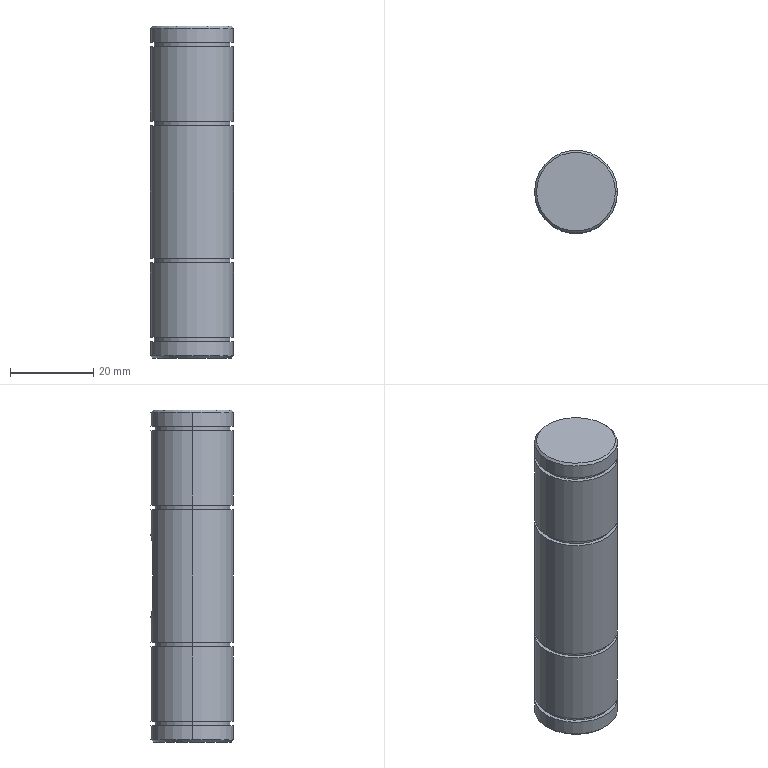Part | STEP file | PN_0015 | 1 solid | 37 faces | box 20 x 20 x 80 mm | volume 24503 mm3 | cylinder 20 | plane 13 | cone 4 | commonest cylinder face diameters 20 x10 18.2 x8 6 x2